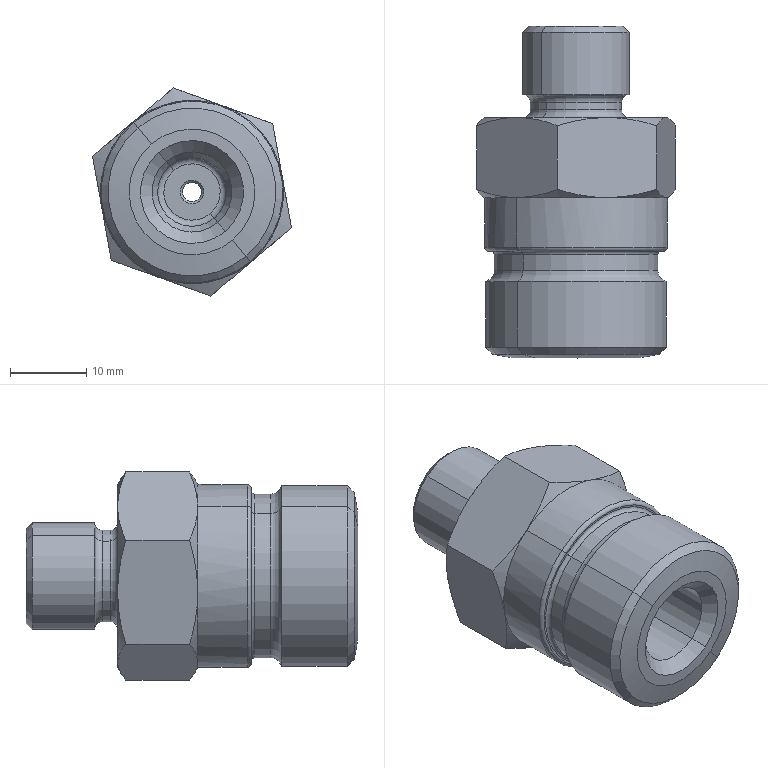Part | SolidWorks | features BaseBody 1 | 1 solid | 67 faces | box 26.081 x 43.5 x 27.271 mm | volume 13876 mm3 | cone 26 | cylinder 16 | torus 14 | plane 11 | commonest cylinder face diameters 2.5 x2 9 x2 10.5 x2 12 x2 14 x2 21.5 x2